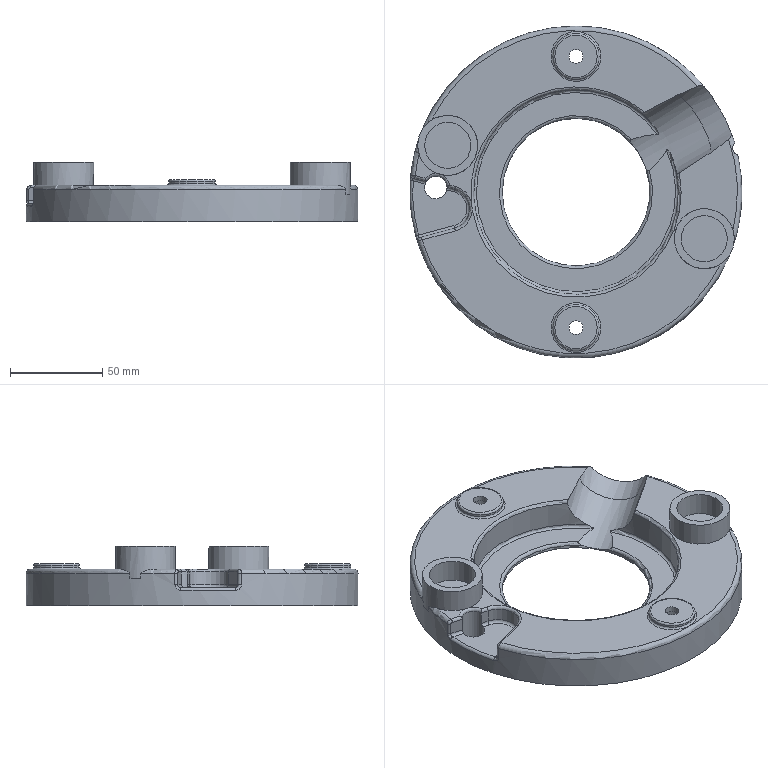Part | STEP file | Base_plate_001 | 1 solid | 76 faces | box 180 x 180 x 32.5 mm | volume 306829 mm3 | cylinder 31 | plane 25 | torus 16 | spline 4 | commonest cylinder face diameters 3 x8 7.5 x6 25 x4 32.5 x4 15.5 x2 8 x1